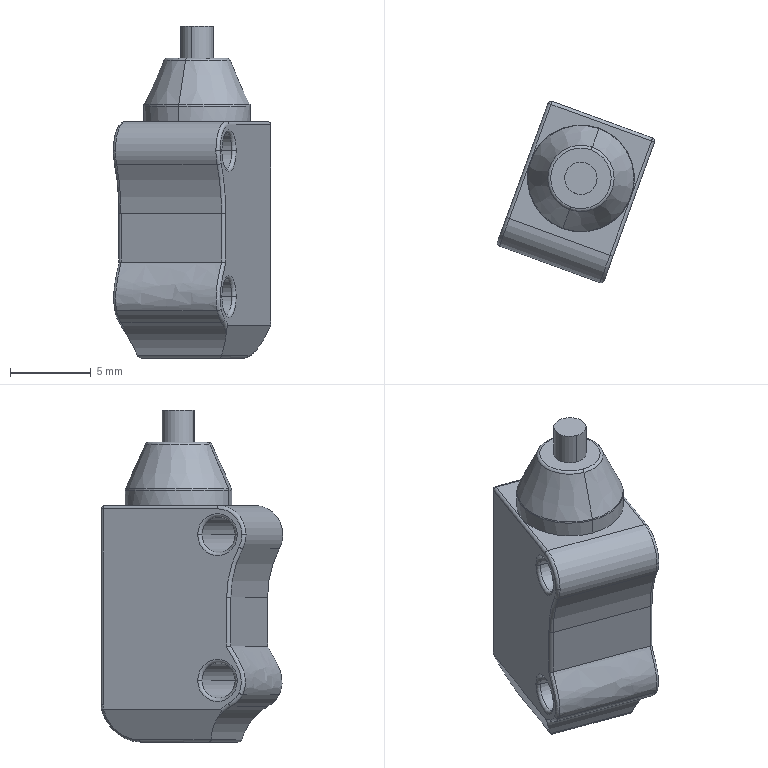Part | SolidWorks | features SplitBody 1 | 1 solid | 76 faces | box 9.714 x 11.209 x 20.5 mm | volume 919.158 mm3 | cylinder 28 | torus 24 | plane 15 | spline 5 | cone 2 | sphere 2 | commonest cylinder face diameters 0.4 x10 2 x4 2.2 x4 4 x3 6.6 x2 3.6 x1